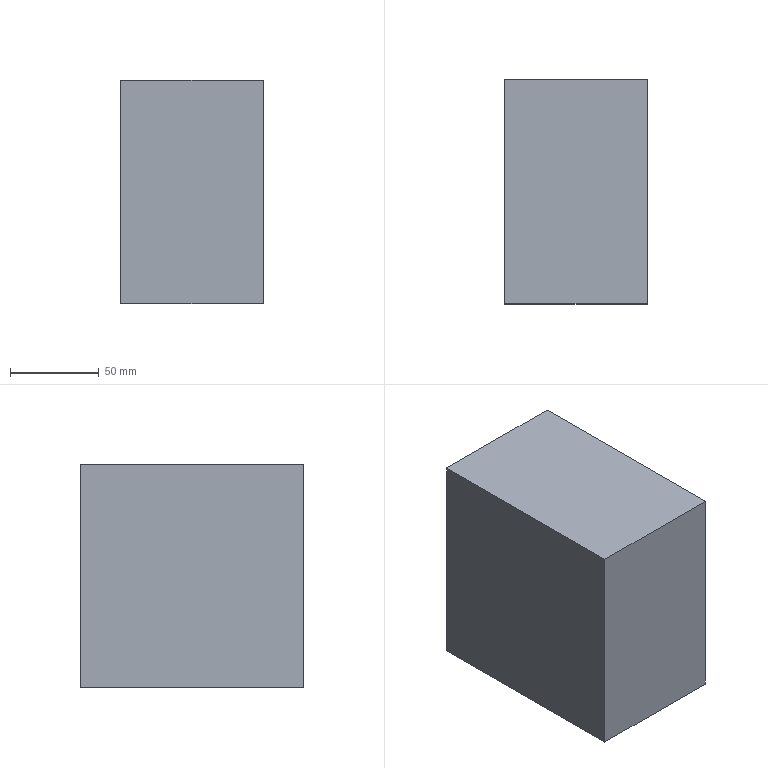Part | SolidWorks | features Extrusion 1, HoleWzd 1 | 1 solid | 14 faces | box 80 x 126 x 126 mm | volume 1136246 mm3 | plane 6 | cylinder 4 | cone 4 | commonest cylinder face diameters 32 x4
STEP:
#1=CARTESIAN_POINT('',(0.,-17.,-50.));
#2=VERTEX_POINT('',#1);
#3=CARTESIAN_POINT('',(0.,-17.,-18.));
#4=VERTEX_POINT('',#3);
#5=CARTESIAN_POINT('',(0.,-17.,-34.));
#6=DIRECTION('',(0.,1.,0.));
#7=DIRECTION('',(0.,0.,1.));
#8=AXIS2_PLACEMENT_3D('',#5,#6,#7);
#9=CIRCLE('',#8,16.);
#10=EDGE_CURVE('',#2,#4,#9,.T.);
#11=ORIENTED_EDGE('',*,*,#10,.F.);
#12=CARTESIAN_POINT('',(0.,63.,-50.));
#13=VERTEX_POINT('',#12);
#14=CARTESIAN_POINT('',(0.,63.,-50.));
#15=DIRECTION('',(0.,1.,0.));
#16=VECTOR('',#15,1000.);
#17=LINE('',#14,#16);
#18=EDGE_CURVE('',#2,#13,#17,.T.);
#19=ORIENTED_EDGE('',*,*,#18,.T.);
#20=CARTESIAN_POINT('',(0.,63.,-18.));
#21=VERTEX_POINT('',#20);
#22=CARTESIAN_POINT('',(0.,63.,-34.));
#23=DIRECTION('',(0.,1.,0.));
#24=DIRECTION('',(0.,0.,1.));
#25=AXIS2_PLACEMENT_3D('',#22,#23,#24);
#26=CIRCLE('',#25,16.);
#27=EDGE_CURVE('',#13,#21,#26,.T.);
#28=ORIENTED_EDGE('',*,*,#27,.T.);
#29=CARTESIAN_POINT('',(0.,63.,-18.));
#30=DIRECTION('',(0.,1.,0.));
#31=VECTOR('',#30,1000.);
#32=LINE('',#29,#31);
#33=EDGE_CURVE('',#4,#21,#32,.T.);
#34=ORIENTED_EDGE('',*,*,#33,.F.);
#35=EDGE_LOOP('',(#11,#19,#28,#34));
#36=FACE_OUTER_BOUND('',#35,.T.);
#37=CARTESIAN_POINT('',(0.,63.,-34.));
#38=DIRECTION('',(0.,1.,0.));
#39=DIRECTION('',(0.,0.,1.));
#40=AXIS2_PLACEMENT_3D('',#37,#38,#39);
#41=CYLINDRICAL_SURFACE('',#40,16.);
#42=ADVANCED_FACE('',(#36),#41,.F.);
#43=CARTESIAN_POINT('',(0.,-26.614,-34.));
#44=VERTEX_POINT('',#43);
#45=CARTESIAN_POINT('',(0.,-17.,-18.));
#46=DIRECTION('',(0.,0.515,0.8572));
#47=VECTOR('',#46,1000.);
#48=LINE('',#45,#47);
#49=EDGE_CURVE('',#44,#4,#48,.T.);
#50=ORIENTED_EDGE('',*,*,#49,.F.);
#51=CARTESIAN_POINT('',(0.,-17.,-50.));
#52=DIRECTION('',(0.,0.515,-0.8572));
#53=VECTOR('',#52,1000.);
#54=LINE('',#51,#53);
#55=EDGE_CURVE('',#44,#2,#54,.T.);
#56=ORIENTED_EDGE('',*,*,#55,.T.);
#57=ORIENTED_EDGE('',*,*,#10,.T.);
#58=EDGE_LOOP('',(#50,#56,#57));
#59=FACE_OUTER_BOUND('',#58,.T.);
#60=CARTESIAN_POINT('',(0.,-17.,-34.));
#61=DIRECTION('',(0.,1.,0.));
#62=DIRECTION('',(0.,0.,1.));
#63=AXIS2_PLACEMENT_3D('',#60,#61,#62);
#64=CONICAL_SURFACE('',#63,16.,1.03);
#65=ADVANCED_FACE('',(#59),#64,.F.);
#66=CARTESIAN_POINT('',(0.,-17.,18.));
#67=VERTEX_POINT('',#66);
#68=CARTESIAN_POINT('',(0.,-17.,50.));
#69=VERTEX_POINT('',#68);
#70=CARTESIAN_POINT('',(0.,-17.,34.));
#71=DIRECTION('',(0.,1.,0.));
#72=DIRECTION('',(0.,0.,1.));
#73=AXIS2_PLACEMENT_3D('',#70,#71,#72);
#74=CIRCLE('',#73,16.);
#75=EDGE_CURVE('',#67,#69,#74,.T.);
#76=ORIENTED_EDGE('',*,*,#75,.F.);
#77=CARTESIAN_POINT('',(0.,63.,18.));
#78=VERTEX_POINT('',#77);
#79=CARTESIAN_POINT('',(0.,63.,18.));
#80=DIRECTION('',(0.,1.,0.));
#81=VECTOR('',#80,1000.);
#82=LINE('',#79,#81);
#83=EDGE_CURVE('',#67,#78,#82,.T.);
#84=ORIENTED_EDGE('',*,*,#83,.T.);
#85=CARTESIAN_POINT('',(0.,63.,50.));
#86=VERTEX_POINT('',#85);
#87=CARTESIAN_POINT('',(0.,63.,34.));
#88=DIRECTION('',(0.,1.,0.));
#89=DIRECTION('',(0.,0.,1.));
#90=AXIS2_PLACEMENT_3D('',#87,#88,#89);
#91=CIRCLE('',#90,16.);
#92=EDGE_CURVE('',#78,#86,#91,.T.);
#93=ORIENTED_EDGE('',*,*,#92,.T.);
#94=CARTESIAN_POINT('',(0.,63.,50.));
#95=DIRECTION('',(0.,1.,0.));
#96=VECTOR('',#95,1000.);
#97=LINE('',#94,#96);
#98=EDGE_CURVE('',#69,#86,#97,.T.);
#99=ORIENTED_EDGE('',*,*,#98,.F.);
#100=EDGE_LOOP('',(#76,#84,#93,#99));
#101=FACE_OUTER_BOUND('',#100,.T.);
#102=CARTESIAN_POINT('',(0.,63.,34.));
#103=DIRECTION('',(0.,1.,0.));
#104=DIRECTION('',(0.,0.,1.));
#105=AXIS2_PLACEMENT_3D('',#102,#103,#104);
#106=CYLINDRICAL_SURFACE('',#105,16.);
#107=ADVANCED_FACE('',(#101),#106,.F.);
#108=CARTESIAN_POINT('',(0.,-26.614,34.));
#109=VERTEX_POINT('',#108);
#110=CARTESIAN_POINT('',(0.,-17.,50.));
#111=DIRECTION('',(0.,0.515,0.8572));
#112=VECTOR('',#111,1000.);
#113=LINE('',#110,#112);
#114=EDGE_CURVE('',#109,#69,#113,.T.);
#115=ORIENTED_EDGE('',*,*,#114,.F.);
#116=CARTESIAN_POINT('',(0.,-17.,18.));
#117=DIRECTION('',(0.,0.515,-0.8572));
#118=VECTOR('',#117,1000.);
#119=LINE('',#116,#118);
#120=EDGE_CURVE('',#109,#67,#119,.T.);
#121=ORIENTED_EDGE('',*,*,#120,.T.);
#122=ORIENTED_EDGE('',*,*,#75,.T.);
#123=EDGE_LOOP('',(#115,#121,#122));
#124=FACE_OUTER_BOUND('',#123,.T.);
#125=CARTESIAN_POINT('',(0.,-17.,34.));
#126=DIRECTION('',(0.,1.,0.));
#127=DIRECTION('',(0.,0.,1.));
#128=AXIS2_PLACEMENT_3D('',#125,#126,#127);
#129=CONICAL_SURFACE('',#128,16.,1.03);
#130=ADVANCED_FACE('',(#124),#129,.F.);
#131=CARTESIAN_POINT('',(-40.,-63.,-63.));
#132=VERTEX_POINT('',#131);
#133=CARTESIAN_POINT('',(-40.,-63.,63.));
#134=VERTEX_POINT('',#133);
#135=CARTESIAN_POINT('',(-40.,-63.,-63.));
#136=DIRECTION('',(0.,0.,1.));
#137=VECTOR('',#136,1000.);
#138=LINE('',#135,#137);
#139=EDGE_CURVE('',#132,#134,#138,.T.);
#140=ORIENTED_EDGE('',*,*,#139,.T.);
#141=CARTESIAN_POINT('',(-40.,63.,63.));
#142=VERTEX_POINT('',#141);
#143=CARTESIAN_POINT('',(-40.,63.,63.));
#144=DIRECTION('',(0.,-1.,0.));
#145=VECTOR('',#144,1000.);
#146=LINE('',#143,#145);
#147=EDGE_CURVE('',#142,#134,#146,.T.);
#148=ORIENTED_EDGE('',*,*,#147,.F.);
#149=CARTESIAN_POINT('',(-40.,63.,-63.));
#150=VERTEX_POINT('',#149);
#151=CARTESIAN_POINT('',(-40.,63.,-63.));
#152=DIRECTION('',(0.,0.,1.));
#153=VECTOR('',#152,1000.);
#154=LINE('',#151,#153);
#155=EDGE_CURVE('',#150,#142,#154,.T.);
#156=ORIENTED_EDGE('',*,*,#155,.F.);
#157=CARTESIAN_POINT('',(-40.,63.,-63.));
#158=DIRECTION('',(0.,-1.,0.));
#159=VECTOR('',#158,1000.);
#160=LINE('',#157,#159);
#161=EDGE_CURVE('',#150,#132,#160,.T.);
#162=ORIENTED_EDGE('',*,*,#161,.T.);
#163=EDGE_LOOP('',(#140,#148,#156,#162));
#164=FACE_OUTER_BOUND('',#163,.T.);
#165=CARTESIAN_POINT('',(-40.,63.,-63.));
#166=DIRECTION('',(1.,0.,0.));
#167=DIRECTION('',(0.,0.,-1.));
#168=AXIS2_PLACEMENT_3D('',#165,#166,#167);
#169=PLANE('',#168);
#170=ADVANCED_FACE('',(#164),#169,.F.);
#171=CARTESIAN_POINT('',(40.,-63.,63.));
#172=VERTEX_POINT('',#171);
#173=CARTESIAN_POINT('',(-40.,-63.,63.));
#174=DIRECTION('',(1.,0.,0.));
#175=VECTOR('',#174,1000.);
#176=LINE('',#173,#175);
#177=EDGE_CURVE('',#134,#172,#176,.T.);
#178=ORIENTED_EDGE('',*,*,#177,.T.);
#179=CARTESIAN_POINT('',(40.,63.,63.));
#180=VERTEX_POINT('',#179);
#181=CARTESIAN_POINT('',(40.,63.,63.));
#182=DIRECTION('',(0.,-1.,0.));
#183=VECTOR('',#182,1000.);
#184=LINE('',#181,#183);
#185=EDGE_CURVE('',#180,#172,#184,.T.);
#186=ORIENTED_EDGE('',*,*,#185,.F.);
#187=CARTESIAN_POINT('',(-40.,63.,63.));
#188=DIRECTION('',(1.,0.,0.));
#189=VECTOR('',#188,1000.);
#190=LINE('',#187,#189);
#191=EDGE_CURVE('',#142,#180,#190,.T.);
#192=ORIENTED_EDGE('',*,*,#191,.F.);
#193=ORIENTED_EDGE('',*,*,#147,.T.);
#194=EDGE_LOOP('',(#178,#186,#192,#193));
#195=FACE_OUTER_BOUND('',#194,.T.);
#196=CARTESIAN_POINT('',(-40.,63.,63.));
#197=DIRECTION('',(0.,0.,-1.));
#198=DIRECTION('',(-1.,0.,0.));
#199=AXIS2_PLACEMENT_3D('',#196,#197,#198);
#200=PLANE('',#199);
#201=ADVANCED_FACE('',(#195),#200,.F.);
#202=CARTESIAN_POINT('',(40.,-63.,-63.));
#203=VERTEX_POINT('',#202);
#204=CARTESIAN_POINT('',(40.,-63.,-63.));
#205=DIRECTION('',(0.,0.,-1.));
#206=VECTOR('',#205,1000.);
#207=LINE('',#204,#206);
#208=EDGE_CURVE('',#172,#203,#207,.T.);
#209=ORIENTED_EDGE('',*,*,#208,.T.);
#210=CARTESIAN_POINT('',(40.,63.,-63.));
#211=VERTEX_POINT('',#210);
#212=CARTESIAN_POINT('',(40.,63.,-63.));
#213=DIRECTION('',(0.,-1.,0.));
#214=VECTOR('',#213,1000.);
#215=LINE('',#212,#214);
#216=EDGE_CURVE('',#211,#203,#215,.T.);
#217=ORIENTED_EDGE('',*,*,#216,.F.);
#218=CARTESIAN_POINT('',(40.,63.,-63.));
#219=DIRECTION('',(0.,0.,-1.));
#220=VECTOR('',#219,1000.);
#221=LINE('',#218,#220);
#222=EDGE_CURVE('',#180,#211,#221,.T.);
#223=ORIENTED_EDGE('',*,*,#222,.F.);
#224=ORIENTED_EDGE('',*,*,#185,.T.);
#225=EDGE_LOOP('',(#209,#217,#223,#224));
#226=FACE_OUTER_BOUND('',#225,.T.);
#227=CARTESIAN_POINT('',(40.,63.,-63.));
#228=DIRECTION('',(-1.,0.,0.));
#229=DIRECTION('',(0.,0.,1.));
#230=AXIS2_PLACEMENT_3D('',#227,#228,#229);
#231=PLANE('',#230);
#232=ADVANCED_FACE('',(#226),#231,.F.);
#233=CARTESIAN_POINT('',(-40.,-63.,-63.));
#234=DIRECTION('',(-1.,0.,0.));
#235=VECTOR('',#234,1000.);
#236=LINE('',#233,#235);
#237=EDGE_CURVE('',#203,#132,#236,.T.);
#238=ORIENTED_EDGE('',*,*,#237,.T.);
#239=ORIENTED_EDGE('',*,*,#161,.F.);
#240=CARTESIAN_POINT('',(-40.,63.,-63.));
#241=DIRECTION('',(-1.,0.,0.));
#242=VECTOR('',#241,1000.);
#243=LINE('',#240,#242);
#244=EDGE_CURVE('',#211,#150,#243,.T.);
#245=ORIENTED_EDGE('',*,*,#244,.F.);
#246=ORIENTED_EDGE('',*,*,#216,.T.);
#247=EDGE_LOOP('',(#238,#239,#245,#246));
#248=FACE_OUTER_BOUND('',#247,.T.);
#249=CARTESIAN_POINT('',(-40.,63.,-63.));
#250=DIRECTION('',(0.,0.,1.));
#251=DIRECTION('',(1.,0.,0.));
#252=AXIS2_PLACEMENT_3D('',#249,#250,#251);
#253=PLANE('',#252);
#254=ADVANCED_FACE('',(#248),#253,.F.);
#255=CARTESIAN_POINT('',(0.,63.,-34.));
#256=DIRECTION('',(0.,1.,0.));
#257=DIRECTION('',(0.,0.,1.));
#258=AXIS2_PLACEMENT_3D('',#255,#256,#257);
#259=CIRCLE('',#258,16.);
#260=EDGE_CURVE('',#21,#13,#259,.T.);
#261=ORIENTED_EDGE('',*,*,#260,.F.);
#262=ORIENTED_EDGE('',*,*,#27,.F.);
#263=EDGE_LOOP('',(#261,#262));
#264=FACE_BOUND('',#263,.T.);
#265=CARTESIAN_POINT('',(0.,63.,34.));
#266=DIRECTION('',(0.,1.,0.));
#267=DIRECTION('',(0.,0.,1.));
#268=AXIS2_PLACEMENT_3D('',#265,#266,#267);
#269=CIRCLE('',#268,16.);
#270=EDGE_CURVE('',#86,#78,#269,.T.);
#271=ORIENTED_EDGE('',*,*,#270,.F.);
#272=ORIENTED_EDGE('',*,*,#92,.F.);
#273=EDGE_LOOP('',(#271,#272));
#274=FACE_BOUND('',#273,.T.);
#275=ORIENTED_EDGE('',*,*,#155,.T.);
#276=ORIENTED_EDGE('',*,*,#191,.T.);
#277=ORIENTED_EDGE('',*,*,#222,.T.);
#278=ORIENTED_EDGE('',*,*,#244,.T.);
#279=EDGE_LOOP('',(#275,#276,#277,#278));
#280=FACE_OUTER_BOUND('',#279,.T.);
#281=CARTESIAN_POINT('',(0.,63.,0.));
#282=DIRECTION('',(0.,1.,0.));
#283=DIRECTION('',(0.,0.,1.));
#284=AXIS2_PLACEMENT_3D('',#281,#282,#283);
#285=PLANE('',#284);
#286=ADVANCED_FACE('',(#264,#274,#280),#285,.T.);
#287=ORIENTED_EDGE('',*,*,#139,.F.);
#288=ORIENTED_EDGE('',*,*,#237,.F.);
#289=ORIENTED_EDGE('',*,*,#208,.F.);
#290=ORIENTED_EDGE('',*,*,#177,.F.);
#291=EDGE_LOOP('',(#287,#288,#289,#290));
#292=FACE_OUTER_BOUND('',#291,.T.);
#293=CARTESIAN_POINT('',(0.,-63.,0.));
#294=DIRECTION('',(0.,1.,0.));
#295=DIRECTION('',(0.,0.,1.));
#296=AXIS2_PLACEMENT_3D('',#293,#294,#295);
#297=PLANE('',#296);
#298=ADVANCED_FACE('',(#292),#297,.F.);
#299=ORIENTED_EDGE('',*,*,#120,.F.);
#300=ORIENTED_EDGE('',*,*,#114,.T.);
#301=CARTESIAN_POINT('',(0.,-17.,34.));
#302=DIRECTION('',(0.,1.,0.));
#303=DIRECTION('',(0.,0.,1.));
#304=AXIS2_PLACEMENT_3D('',#301,#302,#303);
#305=CIRCLE('',#304,16.);
#306=EDGE_CURVE('',#69,#67,#305,.T.);
#307=ORIENTED_EDGE('',*,*,#306,.T.);
#308=EDGE_LOOP('',(#299,#300,#307));
#309=FACE_OUTER_BOUND('',#308,.T.);
#310=CARTESIAN_POINT('',(0.,-17.,34.));
#311=DIRECTION('',(0.,1.,0.));
#312=DIRECTION('',(0.,0.,1.));
#313=AXIS2_PLACEMENT_3D('',#310,#311,#312);
#314=CONICAL_SURFACE('',#313,16.,1.03);
#315=ADVANCED_FACE('',(#309),#314,.F.);
#316=ORIENTED_EDGE('',*,*,#83,.F.);
#317=ORIENTED_EDGE('',*,*,#306,.F.);
#318=ORIENTED_EDGE('',*,*,#98,.T.);
#319=ORIENTED_EDGE('',*,*,#270,.T.);
#320=EDGE_LOOP('',(#316,#317,#318,#319));
#321=FACE_OUTER_BOUND('',#320,.T.);
#322=CARTESIAN_POINT('',(0.,63.,34.));
#323=DIRECTION('',(0.,1.,0.));
#324=DIRECTION('',(0.,0.,1.));
#325=AXIS2_PLACEMENT_3D('',#322,#323,#324);
#326=CYLINDRICAL_SURFACE('',#325,16.);
#327=ADVANCED_FACE('',(#321),#326,.F.);
#328=ORIENTED_EDGE('',*,*,#55,.F.);
#329=ORIENTED_EDGE('',*,*,#49,.T.);
#330=CARTESIAN_POINT('',(0.,-17.,-34.));
#331=DIRECTION('',(0.,1.,0.));
#332=DIRECTION('',(0.,0.,1.));
#333=AXIS2_PLACEMENT_3D('',#330,#331,#332);
#334=CIRCLE('',#333,16.);
#335=EDGE_CURVE('',#4,#2,#334,.T.);
#336=ORIENTED_EDGE('',*,*,#335,.T.);
#337=EDGE_LOOP('',(#328,#329,#336));
#338=FACE_OUTER_BOUND('',#337,.T.);
#339=CARTESIAN_POINT('',(0.,-17.,-34.));
#340=DIRECTION('',(0.,1.,0.));
#341=DIRECTION('',(0.,0.,1.));
#342=AXIS2_PLACEMENT_3D('',#339,#340,#341);
#343=CONICAL_SURFACE('',#342,16.,1.03);
#344=ADVANCED_FACE('',(#338),#343,.F.);
#345=ORIENTED_EDGE('',*,*,#18,.F.);
#346=ORIENTED_EDGE('',*,*,#335,.F.);
#347=ORIENTED_EDGE('',*,*,#33,.T.);
#348=ORIENTED_EDGE('',*,*,#260,.T.);
#349=EDGE_LOOP('',(#345,#346,#347,#348));
#350=FACE_OUTER_BOUND('',#349,.T.);
#351=CARTESIAN_POINT('',(0.,63.,-34.));
#352=DIRECTION('',(0.,1.,0.));
#353=DIRECTION('',(0.,0.,1.));
#354=AXIS2_PLACEMENT_3D('',#351,#352,#353);
#355=CYLINDRICAL_SURFACE('',#354,16.);
#356=ADVANCED_FACE('',(#350),#355,.F.);
#357=CLOSED_SHELL('',(#42,#65,#107,#130,#170,#201,#232,#254,#286,#298,#315,#327,#344,#356));
#358=MANIFOLD_SOLID_BREP('',#357);
#359=CARTESIAN_POINT('',(0.,0.,0.));
#360=DIRECTION('',(0.,0.,1.));
#361=DIRECTION('',(1.,0.,0.));
#362=AXIS2_PLACEMENT_3D('',#359,#360,#361);
#363=(LENGTH_UNIT()NAMED_UNIT(*)SI_UNIT(.MILLI.,.METRE.));
#364=UNCERTAINTY_MEASURE_WITH_UNIT(LENGTH_MEASURE(0.00001),#363,'','');
#365=(NAMED_UNIT(*)PLANE_ANGLE_UNIT()SI_UNIT($,.RADIAN.));
#366=(NAMED_UNIT(*)SI_UNIT($,.STERADIAN.)SOLID_ANGLE_UNIT());
#367=(GEOMETRIC_REPRESENTATION_CONTEXT(3)GLOBAL_UNCERTAINTY_ASSIGNED_CONTEXT((#364))GLOBAL_UNIT_ASSIGNED_CONTEXT((#363,#365,#366))REPRESENTATION_CONTEXT('',''));
#368=ADVANCED_BREP_SHAPE_REPRESENTATION('',(#358,#362),#367);